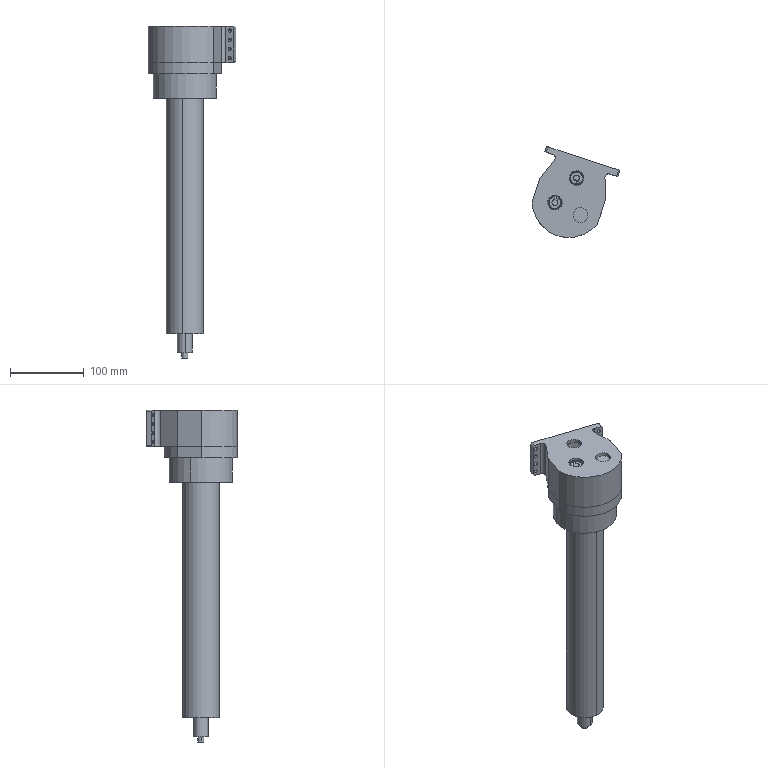Part | SolidWorks | features CompositeCurve 9 | 27 solids | 4409 faces | volume 966521 mm3 | cylinder 1466 | plane 1089 | sphere 1040 | torus 506 | spline 306 | cone 2 | commonest cylinder face diameters 0.475 x273 1.69 x189 0.375 x182 1.689 x84 4 x84 20 x79